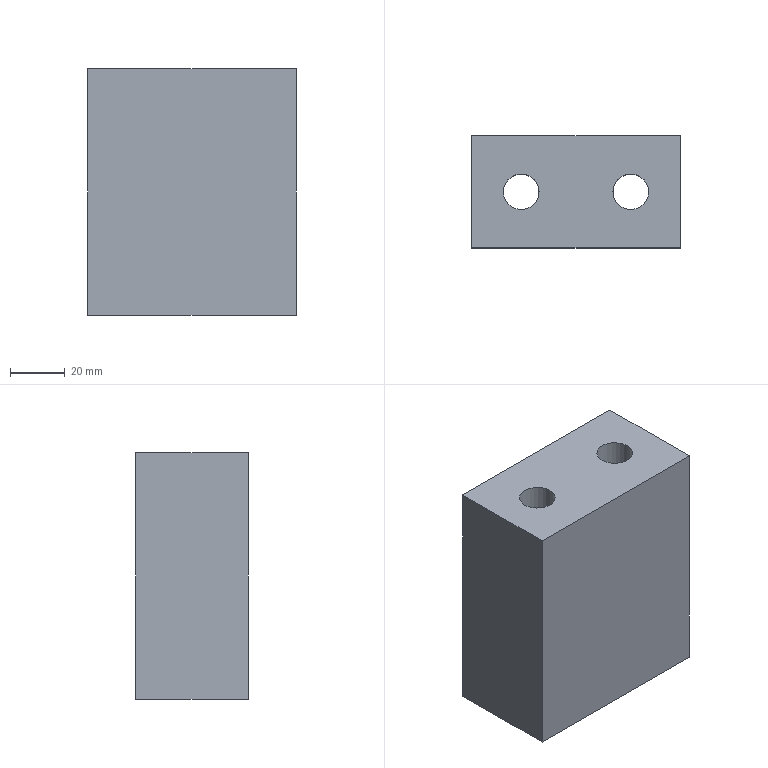Part | STEP file | lll_id3010_x_t | 1 solid | 12 faces | box 76 x 41 x 90 mm | volume 246388 mm3 | plane 8 | cylinder 4 | commonest cylinder face diameters 13 x2 20 x2
STEP:
#1=CARTESIAN_POINT('',(3569.435,287.,52.5));
#2=VERTEX_POINT('',#1);
#3=CARTESIAN_POINT('',(3645.435,287.,52.5));
#4=VERTEX_POINT('',#3);
#5=CARTESIAN_POINT('',(3612.435,287.,52.5));
#6=DIRECTION('',(1.,0.,0.));
#7=VECTOR('',#6,1.);
#8=LINE('',#5,#7);
#9=EDGE_CURVE('',#2,#4,#8,.T.);
#10=ORIENTED_EDGE('',*,*,#9,.F.);
#11=CARTESIAN_POINT('',(3569.435,328.,52.5));
#12=VERTEX_POINT('',#11);
#13=CARTESIAN_POINT('',(3569.435,310.,52.5));
#14=DIRECTION('',(0.,-1.,0.));
#15=VECTOR('',#14,1.);
#16=LINE('',#13,#15);
#17=EDGE_CURVE('',#12,#2,#16,.T.);
#18=ORIENTED_EDGE('',*,*,#17,.F.);
#19=CARTESIAN_POINT('',(3645.435,328.,52.5));
#20=VERTEX_POINT('',#19);
#21=CARTESIAN_POINT('',(3612.435,328.,52.5));
#22=DIRECTION('',(-1.,0.,0.));
#23=VECTOR('',#22,1.);
#24=LINE('',#21,#23);
#25=EDGE_CURVE('',#20,#12,#24,.T.);
#26=ORIENTED_EDGE('',*,*,#25,.F.);
#27=CARTESIAN_POINT('',(3645.435,310.,52.5));
#28=DIRECTION('',(0.,1.,0.));
#29=VECTOR('',#28,1.);
#30=LINE('',#27,#29);
#31=EDGE_CURVE('',#4,#20,#30,.T.);
#32=ORIENTED_EDGE('',*,*,#31,.F.);
#33=EDGE_LOOP('',(#10,#18,#26,#32));
#34=FACE_BOUND('',#33,.T.);
#35=CARTESIAN_POINT('',(3637.435,307.5,52.5));
#36=VERTEX_POINT('',#35);
#37=CARTESIAN_POINT('',(3627.435,307.5,52.5));
#38=DIRECTION('',(0.,0.,-1.));
#39=DIRECTION('',(1.,0.,0.));
#40=AXIS2_PLACEMENT_3D('',#37,#38,#39);
#41=CIRCLE('',#40,10.);
#42=EDGE_CURVE('',#36,#36,#41,.T.);
#43=ORIENTED_EDGE('',*,*,#42,.F.);
#44=EDGE_LOOP('',(#43));
#45=FACE_BOUND('',#44,.T.);
#46=CARTESIAN_POINT('',(3597.435,307.5,52.5));
#47=VERTEX_POINT('',#46);
#48=CARTESIAN_POINT('',(3587.435,307.5,52.5));
#49=DIRECTION('',(0.,0.,1.));
#50=DIRECTION('',(1.,0.,0.));
#51=AXIS2_PLACEMENT_3D('',#48,#49,#50);
#52=CIRCLE('',#51,10.);
#53=EDGE_CURVE('',#47,#47,#52,.T.);
#54=ORIENTED_EDGE('',*,*,#53,.T.);
#55=EDGE_LOOP('',(#54));
#56=FACE_BOUND('',#55,.T.);
#57=CARTESIAN_POINT('',(3612.435,310.,52.5));
#58=DIRECTION('',(0.,0.,-1.));
#59=DIRECTION('',(-1.,0.,0.));
#60=AXIS2_PLACEMENT_3D('',#57,#58,#59);
#61=PLANE('',#60);
#62=ADVANCED_FACE('',(#34,#45,#56),#61,.T.);
#63=CARTESIAN_POINT('',(3580.935,307.5,142.5));
#64=VERTEX_POINT('',#63);
#65=CARTESIAN_POINT('',(3587.435,307.5,142.5));
#66=DIRECTION('',(0.,0.,1.));
#67=DIRECTION('',(-1.,0.,0.));
#68=AXIS2_PLACEMENT_3D('',#65,#66,#67);
#69=CIRCLE('',#68,6.5);
#70=EDGE_CURVE('',#64,#64,#69,.T.);
#71=ORIENTED_EDGE('',*,*,#70,.F.);
#72=EDGE_LOOP('',(#71));
#73=FACE_BOUND('',#72,.T.);
#74=CARTESIAN_POINT('',(3569.435,287.,142.5));
#75=VERTEX_POINT('',#74);
#76=CARTESIAN_POINT('',(3569.435,328.,142.5));
#77=VERTEX_POINT('',#76);
#78=CARTESIAN_POINT('',(3569.435,310.,142.5));
#79=DIRECTION('',(0.,1.,0.));
#80=VECTOR('',#79,1.);
#81=LINE('',#78,#80);
#82=EDGE_CURVE('',#75,#77,#81,.T.);
#83=ORIENTED_EDGE('',*,*,#82,.F.);
#84=CARTESIAN_POINT('',(3645.435,287.,142.5));
#85=VERTEX_POINT('',#84);
#86=CARTESIAN_POINT('',(3612.435,287.,142.5));
#87=DIRECTION('',(-1.,0.,0.));
#88=VECTOR('',#87,1.);
#89=LINE('',#86,#88);
#90=EDGE_CURVE('',#85,#75,#89,.T.);
#91=ORIENTED_EDGE('',*,*,#90,.F.);
#92=CARTESIAN_POINT('',(3645.435,328.,142.5));
#93=VERTEX_POINT('',#92);
#94=CARTESIAN_POINT('',(3645.435,310.,142.5));
#95=DIRECTION('',(0.,-1.,0.));
#96=VECTOR('',#95,1.);
#97=LINE('',#94,#96);
#98=EDGE_CURVE('',#93,#85,#97,.T.);
#99=ORIENTED_EDGE('',*,*,#98,.F.);
#100=CARTESIAN_POINT('',(3612.435,328.,142.5));
#101=DIRECTION('',(1.,0.,0.));
#102=VECTOR('',#101,1.);
#103=LINE('',#100,#102);
#104=EDGE_CURVE('',#77,#93,#103,.T.);
#105=ORIENTED_EDGE('',*,*,#104,.F.);
#106=EDGE_LOOP('',(#83,#91,#99,#105));
#107=FACE_BOUND('',#106,.T.);
#108=CARTESIAN_POINT('',(3620.935,307.5,142.5));
#109=VERTEX_POINT('',#108);
#110=CARTESIAN_POINT('',(3627.435,307.5,142.5));
#111=DIRECTION('',(0.,0.,-1.));
#112=DIRECTION('',(-1.,0.,0.));
#113=AXIS2_PLACEMENT_3D('',#110,#111,#112);
#114=CIRCLE('',#113,6.5);
#115=EDGE_CURVE('',#109,#109,#114,.T.);
#116=ORIENTED_EDGE('',*,*,#115,.T.);
#117=EDGE_LOOP('',(#116));
#118=FACE_BOUND('',#117,.T.);
#119=CARTESIAN_POINT('',(3747.451,598.704,142.5));
#120=DIRECTION('',(0.,0.,1.));
#121=DIRECTION('',(1.,0.,0.));
#122=AXIS2_PLACEMENT_3D('',#119,#120,#121);
#123=PLANE('',#122);
#124=ADVANCED_FACE('',(#73,#107,#118),#123,.T.);
#125=CARTESIAN_POINT('',(3569.435,287.,97.5));
#126=DIRECTION('',(0.,0.,-1.));
#127=VECTOR('',#126,1.);
#128=LINE('',#125,#127);
#129=EDGE_CURVE('',#75,#2,#128,.T.);
#130=ORIENTED_EDGE('',*,*,#129,.T.);
#131=ORIENTED_EDGE('',*,*,#9,.T.);
#132=CARTESIAN_POINT('',(3645.435,287.,97.5));
#133=DIRECTION('',(0.,0.,-1.));
#134=VECTOR('',#133,1.);
#135=LINE('',#132,#134);
#136=EDGE_CURVE('',#85,#4,#135,.T.);
#137=ORIENTED_EDGE('',*,*,#136,.F.);
#138=ORIENTED_EDGE('',*,*,#90,.T.);
#139=EDGE_LOOP('',(#130,#131,#137,#138));
#140=FACE_OUTER_BOUND('',#139,.T.);
#141=CARTESIAN_POINT('',(3612.435,287.,97.5));
#142=DIRECTION('',(0.,-1.,0.));
#143=DIRECTION('',(0.,0.,1.));
#144=AXIS2_PLACEMENT_3D('',#141,#142,#143);
#145=PLANE('',#144);
#146=ADVANCED_FACE('',(#140),#145,.T.);
#147=ORIENTED_EDGE('',*,*,#136,.T.);
#148=ORIENTED_EDGE('',*,*,#31,.T.);
#149=CARTESIAN_POINT('',(3645.435,328.,97.5));
#150=DIRECTION('',(0.,0.,-1.));
#151=VECTOR('',#150,1.);
#152=LINE('',#149,#151);
#153=EDGE_CURVE('',#93,#20,#152,.T.);
#154=ORIENTED_EDGE('',*,*,#153,.F.);
#155=ORIENTED_EDGE('',*,*,#98,.T.);
#156=EDGE_LOOP('',(#147,#148,#154,#155));
#157=FACE_OUTER_BOUND('',#156,.T.);
#158=CARTESIAN_POINT('',(3645.435,310.,97.5));
#159=DIRECTION('',(1.,0.,0.));
#160=DIRECTION('',(0.,0.,-1.));
#161=AXIS2_PLACEMENT_3D('',#158,#159,#160);
#162=PLANE('',#161);
#163=ADVANCED_FACE('',(#157),#162,.T.);
#164=ORIENTED_EDGE('',*,*,#153,.T.);
#165=ORIENTED_EDGE('',*,*,#25,.T.);
#166=CARTESIAN_POINT('',(3569.435,328.,97.5));
#167=DIRECTION('',(0.,0.,-1.));
#168=VECTOR('',#167,1.);
#169=LINE('',#166,#168);
#170=EDGE_CURVE('',#77,#12,#169,.T.);
#171=ORIENTED_EDGE('',*,*,#170,.F.);
#172=ORIENTED_EDGE('',*,*,#104,.T.);
#173=EDGE_LOOP('',(#164,#165,#171,#172));
#174=FACE_OUTER_BOUND('',#173,.T.);
#175=CARTESIAN_POINT('',(3612.435,328.,97.5));
#176=DIRECTION('',(0.,1.,0.));
#177=DIRECTION('',(0.,0.,-1.));
#178=AXIS2_PLACEMENT_3D('',#175,#176,#177);
#179=PLANE('',#178);
#180=ADVANCED_FACE('',(#174),#179,.T.);
#181=ORIENTED_EDGE('',*,*,#82,.T.);
#182=ORIENTED_EDGE('',*,*,#170,.T.);
#183=ORIENTED_EDGE('',*,*,#17,.T.);
#184=ORIENTED_EDGE('',*,*,#129,.F.);
#185=EDGE_LOOP('',(#181,#182,#183,#184));
#186=FACE_OUTER_BOUND('',#185,.T.);
#187=CARTESIAN_POINT('',(3569.435,310.,97.5));
#188=DIRECTION('',(-1.,0.,0.));
#189=DIRECTION('',(0.,0.,1.));
#190=AXIS2_PLACEMENT_3D('',#187,#188,#189);
#191=PLANE('',#190);
#192=ADVANCED_FACE('',(#186),#191,.T.);
#193=CARTESIAN_POINT('',(3617.435,307.5,80.5));
#194=VERTEX_POINT('',#193);
#195=CARTESIAN_POINT('',(3627.435,307.5,80.5));
#196=DIRECTION('',(0.,0.,1.));
#197=DIRECTION('',(-1.,0.,0.));
#198=AXIS2_PLACEMENT_3D('',#195,#196,#197);
#199=CIRCLE('',#198,10.);
#200=EDGE_CURVE('',#194,#194,#199,.T.);
#201=ORIENTED_EDGE('',*,*,#200,.T.);
#202=EDGE_LOOP('',(#201));
#203=FACE_BOUND('',#202,.T.);
#204=ORIENTED_EDGE('',*,*,#42,.T.);
#205=EDGE_LOOP('',(#204));
#206=FACE_BOUND('',#205,.T.);
#207=CARTESIAN_POINT('',(3627.435,307.5,14.3));
#208=DIRECTION('',(0.,0.,1.));
#209=DIRECTION('',(-1.,0.,0.));
#210=AXIS2_PLACEMENT_3D('',#207,#208,#209);
#211=CYLINDRICAL_SURFACE('',#210,10.);
#212=ADVANCED_FACE('',(#203,#206),#211,.F.);
#213=ORIENTED_EDGE('',*,*,#115,.F.);
#214=EDGE_LOOP('',(#213));
#215=FACE_BOUND('',#214,.T.);
#216=CARTESIAN_POINT('',(3620.935,307.5,80.5));
#217=VERTEX_POINT('',#216);
#218=CARTESIAN_POINT('',(3627.435,307.5,80.5));
#219=DIRECTION('',(0.,0.,1.));
#220=DIRECTION('',(-1.,0.,0.));
#221=AXIS2_PLACEMENT_3D('',#218,#219,#220);
#222=CIRCLE('',#221,6.5);
#223=EDGE_CURVE('',#217,#217,#222,.T.);
#224=ORIENTED_EDGE('',*,*,#223,.F.);
#225=EDGE_LOOP('',(#224));
#226=FACE_BOUND('',#225,.T.);
#227=CARTESIAN_POINT('',(3627.435,307.5,114.3));
#228=DIRECTION('',(0.,0.,1.));
#229=DIRECTION('',(-1.,0.,0.));
#230=AXIS2_PLACEMENT_3D('',#227,#228,#229);
#231=CYLINDRICAL_SURFACE('',#230,6.5);
#232=ADVANCED_FACE('',(#215,#226),#231,.F.);
#233=ORIENTED_EDGE('',*,*,#223,.T.);
#234=EDGE_LOOP('',(#233));
#235=FACE_BOUND('',#234,.T.);
#236=ORIENTED_EDGE('',*,*,#200,.F.);
#237=EDGE_LOOP('',(#236));
#238=FACE_BOUND('',#237,.T.);
#239=CARTESIAN_POINT('',(3627.435,307.5,80.5));
#240=DIRECTION('',(0.,0.,1.));
#241=DIRECTION('',(-1.,0.,0.));
#242=AXIS2_PLACEMENT_3D('',#239,#240,#241);
#243=PLANE('',#242);
#244=ADVANCED_FACE('',(#235,#238),#243,.F.);
#245=CARTESIAN_POINT('',(3577.435,307.5,80.5));
#246=VERTEX_POINT('',#245);
#247=CARTESIAN_POINT('',(3587.435,307.5,80.5));
#248=DIRECTION('',(0.,0.,-1.));
#249=DIRECTION('',(-1.,0.,0.));
#250=AXIS2_PLACEMENT_3D('',#247,#248,#249);
#251=CIRCLE('',#250,10.);
#252=EDGE_CURVE('',#246,#246,#251,.T.);
#253=ORIENTED_EDGE('',*,*,#252,.F.);
#254=EDGE_LOOP('',(#253));
#255=FACE_BOUND('',#254,.T.);
#256=ORIENTED_EDGE('',*,*,#53,.F.);
#257=EDGE_LOOP('',(#256));
#258=FACE_BOUND('',#257,.T.);
#259=CARTESIAN_POINT('',(3587.435,307.5,14.3));
#260=DIRECTION('',(0.,0.,1.));
#261=DIRECTION('',(1.,0.,0.));
#262=AXIS2_PLACEMENT_3D('',#259,#260,#261);
#263=CYLINDRICAL_SURFACE('',#262,10.);
#264=ADVANCED_FACE('',(#255,#258),#263,.F.);
#265=ORIENTED_EDGE('',*,*,#70,.T.);
#266=EDGE_LOOP('',(#265));
#267=FACE_BOUND('',#266,.T.);
#268=CARTESIAN_POINT('',(3580.935,307.5,80.5));
#269=VERTEX_POINT('',#268);
#270=CARTESIAN_POINT('',(3587.435,307.5,80.5));
#271=DIRECTION('',(0.,0.,-1.));
#272=DIRECTION('',(-1.,0.,0.));
#273=AXIS2_PLACEMENT_3D('',#270,#271,#272);
#274=CIRCLE('',#273,6.5);
#275=EDGE_CURVE('',#269,#269,#274,.T.);
#276=ORIENTED_EDGE('',*,*,#275,.T.);
#277=EDGE_LOOP('',(#276));
#278=FACE_BOUND('',#277,.T.);
#279=CARTESIAN_POINT('',(3587.435,307.5,114.3));
#280=DIRECTION('',(0.,0.,1.));
#281=DIRECTION('',(1.,0.,0.));
#282=AXIS2_PLACEMENT_3D('',#279,#280,#281);
#283=CYLINDRICAL_SURFACE('',#282,6.5);
#284=ADVANCED_FACE('',(#267,#278),#283,.F.);
#285=ORIENTED_EDGE('',*,*,#275,.F.);
#286=EDGE_LOOP('',(#285));
#287=FACE_BOUND('',#286,.T.);
#288=ORIENTED_EDGE('',*,*,#252,.T.);
#289=EDGE_LOOP('',(#288));
#290=FACE_BOUND('',#289,.T.);
#291=CARTESIAN_POINT('',(3587.435,307.5,80.5));
#292=DIRECTION('',(0.,0.,1.));
#293=DIRECTION('',(1.,0.,0.));
#294=AXIS2_PLACEMENT_3D('',#291,#292,#293);
#295=PLANE('',#294);
#296=ADVANCED_FACE('',(#287,#290),#295,.F.);
#297=CLOSED_SHELL('',(#62,#124,#146,#163,#180,#192,#212,#232,#244,#264,#284,#296));
#298=MANIFOLD_SOLID_BREP('',#297);
#299=(LENGTH_UNIT()NAMED_UNIT(*)SI_UNIT(.MILLI.,.METRE.));
#300=UNCERTAINTY_MEASURE_WITH_UNIT(LENGTH_MEASURE(0.00002),#299,'','');
#301=(NAMED_UNIT(*)PLANE_ANGLE_UNIT()SI_UNIT($,.RADIAN.));
#302=PLANE_ANGLE_MEASURE_WITH_UNIT(PLANE_ANGLE_MEASURE(0.01745),#301);
#303=DIMENSIONAL_EXPONENTS(0.,0.,0.,0.,0.,0.,0.);
#304=(CONVERSION_BASED_UNIT('DEGREE',#302)NAMED_UNIT(#303)PLANE_ANGLE_UNIT());
#305=(NAMED_UNIT(*)SI_UNIT($,.STERADIAN.)SOLID_ANGLE_UNIT());
#306=(GEOMETRIC_REPRESENTATION_CONTEXT(3)GLOBAL_UNCERTAINTY_ASSIGNED_CONTEXT((#300))GLOBAL_UNIT_ASSIGNED_CONTEXT((#299,#304,#305))REPRESENTATION_CONTEXT('',''));
#307=ADVANCED_BREP_SHAPE_REPRESENTATION('',(#298),#306);